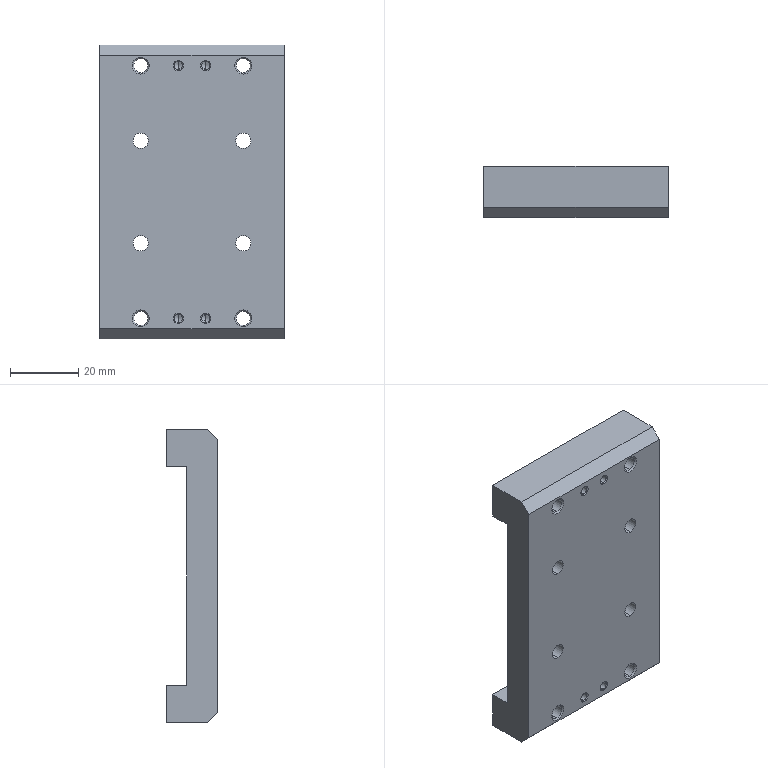Part | STEP file | KR3310A-10A0 carriage | 1 solid | 80 faces | box 54 x 15 x 86 mm | volume 46318 mm3 | cylinder 32 | cone 32 | plane 16 | commonest cylinder face diameters 2.459 x8 4.134 x8 4.5 x8 8 x8